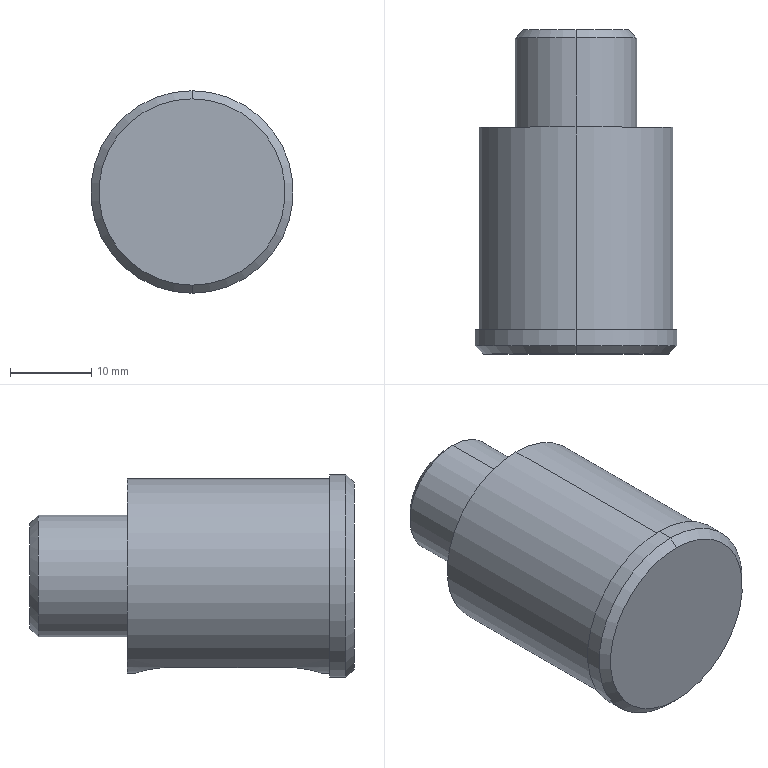Part | SolidWorks | features ICE 3, Chamfer 1, Extrusion 1 | 1 solid | 19 faces | box 25 x 40 x 25 mm | volume 14197 mm3 | cylinder 8 | plane 7 | cone 4 | commonest cylinder face diameters 8 x2 15 x2 24 x2 25 x2
STEP:
#1=CARTESIAN_POINT('',(0.,0.,-11.5));
#2=VERTEX_POINT('',#1);
#3=CARTESIAN_POINT('',(0.,0.,11.5));
#4=VERTEX_POINT('',#3);
#5=CARTESIAN_POINT('',(0.,0.,0.));
#6=DIRECTION('',(0.,-1.,0.));
#7=DIRECTION('',(0.,0.,1.));
#8=AXIS2_PLACEMENT_3D('',#5,#6,#7);
#9=CIRCLE('',#8,11.5);
#10=EDGE_CURVE('',#2,#4,#9,.T.);
#11=ORIENTED_EDGE('',*,*,#10,.F.);
#12=CARTESIAN_POINT('',(0.,1.,-12.5));
#13=VERTEX_POINT('',#12);
#14=CARTESIAN_POINT('',(0.,1.,-12.5));
#15=DIRECTION('',(0.,0.7071,-0.7071));
#16=VECTOR('',#15,1000.);
#17=LINE('',#14,#16);
#18=EDGE_CURVE('',#2,#13,#17,.T.);
#19=ORIENTED_EDGE('',*,*,#18,.T.);
#20=CARTESIAN_POINT('',(0.,1.,12.5));
#21=VERTEX_POINT('',#20);
#22=CARTESIAN_POINT('',(0.,1.,0.));
#23=DIRECTION('',(0.,1.,0.));
#24=DIRECTION('',(0.,0.,1.));
#25=AXIS2_PLACEMENT_3D('',#22,#23,#24);
#26=CIRCLE('',#25,12.5);
#27=EDGE_CURVE('',#21,#13,#26,.T.);
#28=ORIENTED_EDGE('',*,*,#27,.F.);
#29=CARTESIAN_POINT('',(0.,1.,12.5));
#30=DIRECTION('',(0.,0.7071,0.7071));
#31=VECTOR('',#30,1000.);
#32=LINE('',#29,#31);
#33=EDGE_CURVE('',#4,#21,#32,.T.);
#34=ORIENTED_EDGE('',*,*,#33,.F.);
#35=EDGE_LOOP('',(#11,#19,#28,#34));
#36=FACE_OUTER_BOUND('',#35,.T.);
#37=CARTESIAN_POINT('',(0.,1.,0.));
#38=DIRECTION('',(0.,1.,0.));
#39=DIRECTION('',(0.,0.,1.));
#40=AXIS2_PLACEMENT_3D('',#37,#38,#39);
#41=CONICAL_SURFACE('',#40,12.5,0.7854);
#42=ADVANCED_FACE('',(#36),#41,.T.);
#43=CARTESIAN_POINT('',(0.,40.,6.5));
#44=VERTEX_POINT('',#43);
#45=CARTESIAN_POINT('',(0.,40.,-6.5));
#46=VERTEX_POINT('',#45);
#47=CARTESIAN_POINT('',(0.,40.,0.));
#48=DIRECTION('',(0.,1.,0.));
#49=DIRECTION('',(0.,0.,1.));
#50=AXIS2_PLACEMENT_3D('',#47,#48,#49);
#51=CIRCLE('',#50,6.5);
#52=EDGE_CURVE('',#44,#46,#51,.T.);
#53=ORIENTED_EDGE('',*,*,#52,.F.);
#54=CARTESIAN_POINT('',(0.,39.,7.5));
#55=VERTEX_POINT('',#54);
#56=CARTESIAN_POINT('',(0.,40.,6.5));
#57=DIRECTION('',(0.,-0.7071,0.7071));
#58=VECTOR('',#57,1000.);
#59=LINE('',#56,#58);
#60=EDGE_CURVE('',#44,#55,#59,.T.);
#61=ORIENTED_EDGE('',*,*,#60,.T.);
#62=CARTESIAN_POINT('',(0.,39.,-7.5));
#63=VERTEX_POINT('',#62);
#64=CARTESIAN_POINT('',(0.,39.,0.));
#65=DIRECTION('',(0.,-1.,0.));
#66=DIRECTION('',(0.,0.,1.));
#67=AXIS2_PLACEMENT_3D('',#64,#65,#66);
#68=CIRCLE('',#67,7.5);
#69=EDGE_CURVE('',#63,#55,#68,.T.);
#70=ORIENTED_EDGE('',*,*,#69,.F.);
#71=CARTESIAN_POINT('',(0.,40.,-6.5));
#72=DIRECTION('',(0.,-0.7071,-0.7071));
#73=VECTOR('',#72,1000.);
#74=LINE('',#71,#73);
#75=EDGE_CURVE('',#46,#63,#74,.T.);
#76=ORIENTED_EDGE('',*,*,#75,.F.);
#77=EDGE_LOOP('',(#53,#61,#70,#76));
#78=FACE_OUTER_BOUND('',#77,.T.);
#79=CARTESIAN_POINT('',(0.,40.,0.));
#80=DIRECTION('',(0.,-1.,0.));
#81=DIRECTION('',(0.,0.,-1.));
#82=AXIS2_PLACEMENT_3D('',#79,#80,#81);
#83=CONICAL_SURFACE('',#82,6.5,0.7854);
#84=ADVANCED_FACE('',(#78),#83,.T.);
#85=ORIENTED_EDGE('',*,*,#69,.T.);
#86=CARTESIAN_POINT('',(0.,28.,7.5));
#87=VERTEX_POINT('',#86);
#88=CARTESIAN_POINT('',(0.,40.,7.5));
#89=DIRECTION('',(0.,-1.,0.));
#90=VECTOR('',#89,1000.);
#91=LINE('',#88,#90);
#92=EDGE_CURVE('',#55,#87,#91,.T.);
#93=ORIENTED_EDGE('',*,*,#92,.T.);
#94=CARTESIAN_POINT('',(0.,28.,-7.5));
#95=VERTEX_POINT('',#94);
#96=CARTESIAN_POINT('',(0.,28.,0.));
#97=DIRECTION('',(0.,1.,0.));
#98=DIRECTION('',(0.,0.,1.));
#99=AXIS2_PLACEMENT_3D('',#96,#97,#98);
#100=CIRCLE('',#99,7.5);
#101=EDGE_CURVE('',#87,#95,#100,.T.);
#102=ORIENTED_EDGE('',*,*,#101,.T.);
#103=CARTESIAN_POINT('',(0.,40.,-7.5));
#104=DIRECTION('',(0.,-1.,0.));
#105=VECTOR('',#104,1000.);
#106=LINE('',#103,#105);
#107=EDGE_CURVE('',#63,#95,#106,.T.);
#108=ORIENTED_EDGE('',*,*,#107,.F.);
#109=EDGE_LOOP('',(#85,#93,#102,#108));
#110=FACE_OUTER_BOUND('',#109,.T.);
#111=CARTESIAN_POINT('',(0.,40.,0.));
#112=DIRECTION('',(0.,-1.,0.));
#113=DIRECTION('',(0.,0.,-1.));
#114=AXIS2_PLACEMENT_3D('',#111,#112,#113);
#115=CYLINDRICAL_SURFACE('',#114,7.5);
#116=ADVANCED_FACE('',(#110),#115,.T.);
#117=CARTESIAN_POINT('',(0.,28.,12.));
#118=VERTEX_POINT('',#117);
#119=CARTESIAN_POINT('',(0.,28.,-12.));
#120=VERTEX_POINT('',#119);
#121=CARTESIAN_POINT('',(0.,28.,0.));
#122=DIRECTION('',(0.,1.,0.));
#123=DIRECTION('',(0.,0.,1.));
#124=AXIS2_PLACEMENT_3D('',#121,#122,#123);
#125=CIRCLE('',#124,12.);
#126=EDGE_CURVE('',#118,#120,#125,.T.);
#127=ORIENTED_EDGE('',*,*,#126,.F.);
#128=CARTESIAN_POINT('',(0.,3.,12.));
#129=VERTEX_POINT('',#128);
#130=CARTESIAN_POINT('',(0.,28.,12.));
#131=DIRECTION('',(0.,-1.,0.));
#132=VECTOR('',#131,1000.);
#133=LINE('',#130,#132);
#134=EDGE_CURVE('',#118,#129,#133,.T.);
#135=ORIENTED_EDGE('',*,*,#134,.T.);
#136=CARTESIAN_POINT('',(0.,3.,-12.));
#137=VERTEX_POINT('',#136);
#138=CARTESIAN_POINT('',(0.,3.,0.));
#139=DIRECTION('',(0.,1.,0.));
#140=DIRECTION('',(0.,0.,1.));
#141=AXIS2_PLACEMENT_3D('',#138,#139,#140);
#142=CIRCLE('',#141,12.);
#143=EDGE_CURVE('',#129,#137,#142,.T.);
#144=ORIENTED_EDGE('',*,*,#143,.T.);
#145=CARTESIAN_POINT('',(0.,4.,-12.));
#146=VERTEX_POINT('',#145);
#147=CARTESIAN_POINT('',(0.,28.,-12.));
#148=DIRECTION('',(0.,-1.,0.));
#149=VECTOR('',#148,1000.);
#150=LINE('',#147,#149);
#151=EDGE_CURVE('',#146,#137,#150,.T.);
#152=ORIENTED_EDGE('',*,*,#151,.F.);
#153=CARTESIAN_POINT('',(4.,8.,-11.314));
#154=VERTEX_POINT('',#153);
#155=CARTESIAN_POINT('',(0.,4.,-12.));
#156=CARTESIAN_POINT('',(0.2628,4.,-12.));
#157=CARTESIAN_POINT('',(0.5297,4.027,-11.991));
#158=CARTESIAN_POINT('',(1.044,4.13,-11.957));
#159=CARTESIAN_POINT('',(1.294,4.206,-11.933));
#160=CARTESIAN_POINT('',(1.78,4.408,-11.87));
#161=CARTESIAN_POINT('',(2.011,4.533,-11.832));
#162=CARTESIAN_POINT('',(2.442,4.821,-11.751));
#163=CARTESIAN_POINT('',(2.645,4.988,-11.706));
#164=CARTESIAN_POINT('',(3.013,5.356,-11.617));
#165=CARTESIAN_POINT('',(3.177,5.556,-11.573));
#166=CARTESIAN_POINT('',(3.467,5.987,-11.489));
#167=CARTESIAN_POINT('',(3.592,6.221,-11.45));
#168=CARTESIAN_POINT('',(3.792,6.702,-11.385));
#169=CARTESIAN_POINT('',(3.869,6.951,-11.359));
#170=CARTESIAN_POINT('',(3.973,7.468,-11.323));
#171=CARTESIAN_POINT('',(4.,7.734,-11.314));
#172=CARTESIAN_POINT('',(4.,8.,-11.314));
#173=B_SPLINE_CURVE_WITH_KNOTS('',3,(#155,#156,#157,#158,#159,#160,#161,#162,#163,#164,#165,#166,#167,#168,#169,#170,#171,#172),.UNSPECIFIED.,.F.,.F.,(4,2,2,2,2,2,2,2,4),(0.0063,0.007086,0.007873,0.008659,0.009446,0.01023,0.01102,0.01181,0.01259),.UNSPECIFIED.);
#174=EDGE_CURVE('',#146,#154,#173,.T.);
#175=ORIENTED_EDGE('',*,*,#174,.T.);
#176=CARTESIAN_POINT('',(4.,23.,-11.314));
#177=VERTEX_POINT('',#176);
#178=CARTESIAN_POINT('',(4.,28.,-11.314));
#179=DIRECTION('',(0.,1.,0.));
#180=VECTOR('',#179,1000.);
#181=LINE('',#178,#180);
#182=EDGE_CURVE('',#154,#177,#181,.T.);
#183=ORIENTED_EDGE('',*,*,#182,.T.);
#184=CARTESIAN_POINT('',(0.,27.,-12.));
#185=VERTEX_POINT('',#184);
#186=CARTESIAN_POINT('',(4.,23.,-11.314));
#187=CARTESIAN_POINT('',(4.,23.266,-11.314));
#188=CARTESIAN_POINT('',(3.974,23.528,-11.323));
#189=CARTESIAN_POINT('',(3.871,24.042,-11.359));
#190=CARTESIAN_POINT('',(3.793,24.297,-11.385));
#191=CARTESIAN_POINT('',(3.591,24.781,-11.45));
#192=CARTESIAN_POINT('',(3.468,25.01,-11.489));
#193=CARTESIAN_POINT('',(3.178,25.443,-11.573));
#194=CARTESIAN_POINT('',(3.01,25.647,-11.618));
#195=CARTESIAN_POINT('',(2.644,26.013,-11.707));
#196=CARTESIAN_POINT('',(2.444,26.178,-11.751));
#197=CARTESIAN_POINT('',(2.007,26.47,-11.833));
#198=CARTESIAN_POINT('',(1.777,26.593,-11.87));
#199=CARTESIAN_POINT('',(1.296,26.793,-11.932));
#200=CARTESIAN_POINT('',(1.042,26.871,-11.958));
#201=CARTESIAN_POINT('',(0.5242,26.974,-11.991));
#202=CARTESIAN_POINT('',(0.2632,27.,-12.));
#203=CARTESIAN_POINT('',(0.,27.,-12.));
#204=B_SPLINE_CURVE_WITH_KNOTS('',3,(#186,#187,#188,#189,#190,#191,#192,#193,#194,#195,#196,#197,#198,#199,#200,#201,#202,#203),.UNSPECIFIED.,.F.,.F.,(4,2,2,2,2,2,2,2,4),(0.,0.0007875,0.001575,0.002362,0.00315,0.003937,0.004725,0.005512,0.0063),.UNSPECIFIED.);
#205=EDGE_CURVE('',#177,#185,#204,.T.);
#206=ORIENTED_EDGE('',*,*,#205,.T.);
#207=CARTESIAN_POINT('',(0.,28.,-12.));
#208=DIRECTION('',(0.,-1.,0.));
#209=VECTOR('',#208,1000.);
#210=LINE('',#207,#209);
#211=EDGE_CURVE('',#120,#185,#210,.T.);
#212=ORIENTED_EDGE('',*,*,#211,.F.);
#213=EDGE_LOOP('',(#127,#135,#144,#152,#175,#183,#206,#212));
#214=FACE_OUTER_BOUND('',#213,.T.);
#215=CARTESIAN_POINT('',(0.,28.,0.));
#216=DIRECTION('',(0.,-1.,0.));
#217=DIRECTION('',(0.,0.,-1.));
#218=AXIS2_PLACEMENT_3D('',#215,#216,#217);
#219=CYLINDRICAL_SURFACE('',#218,12.);
#220=ADVANCED_FACE('',(#214),#219,.T.);
#221=CARTESIAN_POINT('',(0.,3.,12.5));
#222=VERTEX_POINT('',#221);
#223=CARTESIAN_POINT('',(0.,3.,-12.5));
#224=VERTEX_POINT('',#223);
#225=CARTESIAN_POINT('',(0.,3.,0.));
#226=DIRECTION('',(0.,1.,0.));
#227=DIRECTION('',(0.,0.,1.));
#228=AXIS2_PLACEMENT_3D('',#225,#226,#227);
#229=CIRCLE('',#228,12.5);
#230=EDGE_CURVE('',#222,#224,#229,.T.);
#231=ORIENTED_EDGE('',*,*,#230,.F.);
#232=CARTESIAN_POINT('',(0.,3.,12.5));
#233=DIRECTION('',(0.,-1.,0.));
#234=VECTOR('',#233,1000.);
#235=LINE('',#232,#234);
#236=EDGE_CURVE('',#222,#21,#235,.T.);
#237=ORIENTED_EDGE('',*,*,#236,.T.);
#238=ORIENTED_EDGE('',*,*,#27,.T.);
#239=CARTESIAN_POINT('',(0.,3.,-12.5));
#240=DIRECTION('',(0.,-1.,0.));
#241=VECTOR('',#240,1000.);
#242=LINE('',#239,#241);
#243=EDGE_CURVE('',#224,#13,#242,.T.);
#244=ORIENTED_EDGE('',*,*,#243,.F.);
#245=EDGE_LOOP('',(#231,#237,#238,#244));
#246=FACE_OUTER_BOUND('',#245,.T.);
#247=CARTESIAN_POINT('',(0.,3.,0.));
#248=DIRECTION('',(0.,-1.,0.));
#249=DIRECTION('',(0.,0.,-1.));
#250=AXIS2_PLACEMENT_3D('',#247,#248,#249);
#251=CYLINDRICAL_SURFACE('',#250,12.5);
#252=ADVANCED_FACE('',(#246),#251,.T.);
#253=ORIENTED_EDGE('',*,*,#236,.F.);
#254=CARTESIAN_POINT('',(0.,3.,0.));
#255=DIRECTION('',(0.,1.,0.));
#256=DIRECTION('',(0.,0.,1.));
#257=AXIS2_PLACEMENT_3D('',#254,#255,#256);
#258=CIRCLE('',#257,12.5);
#259=EDGE_CURVE('',#224,#222,#258,.T.);
#260=ORIENTED_EDGE('',*,*,#259,.F.);
#261=ORIENTED_EDGE('',*,*,#243,.T.);
#262=CARTESIAN_POINT('',(0.,1.,0.));
#263=DIRECTION('',(0.,1.,0.));
#264=DIRECTION('',(0.,0.,1.));
#265=AXIS2_PLACEMENT_3D('',#262,#263,#264);
#266=CIRCLE('',#265,12.5);
#267=EDGE_CURVE('',#13,#21,#266,.T.);
#268=ORIENTED_EDGE('',*,*,#267,.T.);
#269=EDGE_LOOP('',(#253,#260,#261,#268));
#270=FACE_OUTER_BOUND('',#269,.T.);
#271=CARTESIAN_POINT('',(0.,3.,0.));
#272=DIRECTION('',(0.,-1.,0.));
#273=DIRECTION('',(0.,0.,-1.));
#274=AXIS2_PLACEMENT_3D('',#271,#272,#273);
#275=CYLINDRICAL_SURFACE('',#274,12.5);
#276=ADVANCED_FACE('',(#270),#275,.T.);
#277=CARTESIAN_POINT('',(0.,3.,0.));
#278=DIRECTION('',(0.,1.,0.));
#279=DIRECTION('',(0.,0.,1.));
#280=AXIS2_PLACEMENT_3D('',#277,#278,#279);
#281=CIRCLE('',#280,12.);
#282=EDGE_CURVE('',#137,#129,#281,.T.);
#283=ORIENTED_EDGE('',*,*,#282,.F.);
#284=ORIENTED_EDGE('',*,*,#143,.F.);
#285=EDGE_LOOP('',(#283,#284));
#286=FACE_BOUND('',#285,.T.);
#287=ORIENTED_EDGE('',*,*,#259,.T.);
#288=ORIENTED_EDGE('',*,*,#230,.T.);
#289=EDGE_LOOP('',(#287,#288));
#290=FACE_OUTER_BOUND('',#289,.T.);
#291=CARTESIAN_POINT('',(0.,3.,0.));
#292=DIRECTION('',(0.,1.,0.));
#293=DIRECTION('',(0.,0.,1.));
#294=AXIS2_PLACEMENT_3D('',#291,#292,#293);
#295=PLANE('',#294);
#296=ADVANCED_FACE('',(#286,#290),#295,.T.);
#297=CARTESIAN_POINT('',(0.,0.,0.));
#298=DIRECTION('',(0.,-1.,0.));
#299=DIRECTION('',(0.,0.,1.));
#300=AXIS2_PLACEMENT_3D('',#297,#298,#299);
#301=CIRCLE('',#300,11.5);
#302=EDGE_CURVE('',#4,#2,#301,.T.);
#303=ORIENTED_EDGE('',*,*,#302,.T.);
#304=ORIENTED_EDGE('',*,*,#10,.T.);
#305=EDGE_LOOP('',(#303,#304));
#306=FACE_OUTER_BOUND('',#305,.T.);
#307=CARTESIAN_POINT('',(0.,0.,0.));
#308=DIRECTION('',(0.,1.,0.));
#309=DIRECTION('',(0.,0.,1.));
#310=AXIS2_PLACEMENT_3D('',#307,#308,#309);
#311=PLANE('',#310);
#312=ADVANCED_FACE('',(#306),#311,.F.);
#313=ORIENTED_EDGE('',*,*,#134,.F.);
#314=CARTESIAN_POINT('',(0.,28.,0.));
#315=DIRECTION('',(0.,1.,0.));
#316=DIRECTION('',(0.,0.,1.));
#317=AXIS2_PLACEMENT_3D('',#314,#315,#316);
#318=CIRCLE('',#317,12.);
#319=EDGE_CURVE('',#120,#118,#318,.T.);
#320=ORIENTED_EDGE('',*,*,#319,.F.);
#321=ORIENTED_EDGE('',*,*,#211,.T.);
#322=CARTESIAN_POINT('',(-4.,23.,-11.314));
#323=VERTEX_POINT('',#322);
#324=CARTESIAN_POINT('',(0.,27.,-12.));
#325=CARTESIAN_POINT('',(-0.2628,27.,-12.));
#326=CARTESIAN_POINT('',(-0.5297,26.973,-11.991));
#327=CARTESIAN_POINT('',(-1.044,26.87,-11.957));
#328=CARTESIAN_POINT('',(-1.294,26.794,-11.933));
#329=CARTESIAN_POINT('',(-1.78,26.592,-11.87));
#330=CARTESIAN_POINT('',(-2.011,26.467,-11.832));
#331=CARTESIAN_POINT('',(-2.442,26.179,-11.751));
#332=CARTESIAN_POINT('',(-2.645,26.012,-11.706));
#333=CARTESIAN_POINT('',(-3.013,25.644,-11.617));
#334=CARTESIAN_POINT('',(-3.177,25.444,-11.573));
#335=CARTESIAN_POINT('',(-3.467,25.013,-11.489));
#336=CARTESIAN_POINT('',(-3.592,24.779,-11.45));
#337=CARTESIAN_POINT('',(-3.792,24.298,-11.385));
#338=CARTESIAN_POINT('',(-3.869,24.049,-11.359));
#339=CARTESIAN_POINT('',(-3.973,23.532,-11.323));
#340=CARTESIAN_POINT('',(-4.,23.266,-11.314));
#341=CARTESIAN_POINT('',(-4.,23.,-11.314));
#342=B_SPLINE_CURVE_WITH_KNOTS('',3,(#324,#325,#326,#327,#328,#329,#330,#331,#332,#333,#334,#335,#336,#337,#338,#339,#340,#341),.UNSPECIFIED.,.F.,.F.,(4,2,2,2,2,2,2,2,4),(0.0063,0.007086,0.007873,0.008659,0.009446,0.01023,0.01102,0.01181,0.01259),.UNSPECIFIED.);
#343=EDGE_CURVE('',#185,#323,#342,.T.);
#344=ORIENTED_EDGE('',*,*,#343,.T.);
#345=CARTESIAN_POINT('',(-4.,8.,-11.314));
#346=VERTEX_POINT('',#345);
#347=CARTESIAN_POINT('',(-4.,28.,-11.314));
#348=DIRECTION('',(0.,-1.,0.));
#349=VECTOR('',#348,1000.);
#350=LINE('',#347,#349);
#351=EDGE_CURVE('',#323,#346,#350,.T.);
#352=ORIENTED_EDGE('',*,*,#351,.T.);
#353=CARTESIAN_POINT('',(-4.,8.,-11.314));
#354=CARTESIAN_POINT('',(-4.,7.734,-11.314));
#355=CARTESIAN_POINT('',(-3.974,7.472,-11.323));
#356=CARTESIAN_POINT('',(-3.871,6.958,-11.359));
#357=CARTESIAN_POINT('',(-3.793,6.703,-11.385));
#358=CARTESIAN_POINT('',(-3.591,6.219,-11.45));
#359=CARTESIAN_POINT('',(-3.468,5.99,-11.489));
#360=CARTESIAN_POINT('',(-3.178,5.557,-11.573));
#361=CARTESIAN_POINT('',(-3.01,5.353,-11.618));
#362=CARTESIAN_POINT('',(-2.644,4.987,-11.707));
#363=CARTESIAN_POINT('',(-2.444,4.822,-11.751));
#364=CARTESIAN_POINT('',(-2.007,4.53,-11.833));
#365=CARTESIAN_POINT('',(-1.777,4.407,-11.87));
#366=CARTESIAN_POINT('',(-1.296,4.207,-11.932));
#367=CARTESIAN_POINT('',(-1.042,4.129,-11.958));
#368=CARTESIAN_POINT('',(-0.5242,4.026,-11.991));
#369=CARTESIAN_POINT('',(-0.2632,4.,-12.));
#370=CARTESIAN_POINT('',(0.,4.,-12.));
#371=B_SPLINE_CURVE_WITH_KNOTS('',3,(#353,#354,#355,#356,#357,#358,#359,#360,#361,#362,#363,#364,#365,#366,#367,#368,#369,#370),.UNSPECIFIED.,.F.,.F.,(4,2,2,2,2,2,2,2,4),(0.,0.0007875,0.001575,0.002362,0.00315,0.003937,0.004725,0.005512,0.0063),.UNSPECIFIED.);
#372=EDGE_CURVE('',#346,#146,#371,.T.);
#373=ORIENTED_EDGE('',*,*,#372,.T.);
#374=ORIENTED_EDGE('',*,*,#151,.T.);
#375=ORIENTED_EDGE('',*,*,#282,.T.);
#376=EDGE_LOOP('',(#313,#320,#321,#344,#352,#373,#374,#375));
#377=FACE_OUTER_BOUND('',#376,.T.);
#378=CARTESIAN_POINT('',(0.,28.,0.));
#379=DIRECTION('',(0.,-1.,0.));
#380=DIRECTION('',(0.,0.,-1.));
#381=AXIS2_PLACEMENT_3D('',#378,#379,#380);
#382=CYLINDRICAL_SURFACE('',#381,12.);
#383=ADVANCED_FACE('',(#377),#382,.T.);
#384=CARTESIAN_POINT('',(0.,28.,0.));
#385=DIRECTION('',(0.,1.,0.));
#386=DIRECTION('',(0.,0.,1.));
#387=AXIS2_PLACEMENT_3D('',#384,#385,#386);
#388=CIRCLE('',#387,7.5);
#389=EDGE_CURVE('',#95,#87,#388,.T.);
#390=ORIENTED_EDGE('',*,*,#389,.F.);
#391=ORIENTED_EDGE('',*,*,#101,.F.);
#392=EDGE_LOOP('',(#390,#391));
#393=FACE_BOUND('',#392,.T.);
#394=ORIENTED_EDGE('',*,*,#319,.T.);
#395=ORIENTED_EDGE('',*,*,#126,.T.);
#396=EDGE_LOOP('',(#394,#395));
#397=FACE_OUTER_BOUND('',#396,.T.);
#398=CARTESIAN_POINT('',(0.,28.,0.));
#399=DIRECTION('',(0.,1.,0.));
#400=DIRECTION('',(0.,0.,1.));
#401=AXIS2_PLACEMENT_3D('',#398,#399,#400);
#402=PLANE('',#401);
#403=ADVANCED_FACE('',(#393,#397),#402,.T.);
#404=ORIENTED_EDGE('',*,*,#92,.F.);
#405=CARTESIAN_POINT('',(0.,39.,0.));
#406=DIRECTION('',(0.,-1.,0.));
#407=DIRECTION('',(0.,0.,1.));
#408=AXIS2_PLACEMENT_3D('',#405,#406,#407);
#409=CIRCLE('',#408,7.5);
#410=EDGE_CURVE('',#55,#63,#409,.T.);
#411=ORIENTED_EDGE('',*,*,#410,.T.);
#412=ORIENTED_EDGE('',*,*,#107,.T.);
#413=ORIENTED_EDGE('',*,*,#389,.T.);
#414=EDGE_LOOP('',(#404,#411,#412,#413));
#415=FACE_OUTER_BOUND('',#414,.T.);
#416=CARTESIAN_POINT('',(0.,40.,0.));
#417=DIRECTION('',(0.,-1.,0.));
#418=DIRECTION('',(0.,0.,-1.));
#419=AXIS2_PLACEMENT_3D('',#416,#417,#418);
#420=CYLINDRICAL_SURFACE('',#419,7.5);
#421=ADVANCED_FACE('',(#415),#420,.T.);
#422=CARTESIAN_POINT('',(0.,40.,0.));
#423=DIRECTION('',(0.,1.,0.));
#424=DIRECTION('',(0.,0.,1.));
#425=AXIS2_PLACEMENT_3D('',#422,#423,#424);
#426=CIRCLE('',#425,6.5);
#427=EDGE_CURVE('',#46,#44,#426,.T.);
#428=ORIENTED_EDGE('',*,*,#427,.T.);
#429=ORIENTED_EDGE('',*,*,#52,.T.);
#430=EDGE_LOOP('',(#428,#429));
#431=FACE_OUTER_BOUND('',#430,.T.);
#432=CARTESIAN_POINT('',(0.,40.,0.));
#433=DIRECTION('',(0.,1.,0.));
#434=DIRECTION('',(0.,0.,1.));
#435=AXIS2_PLACEMENT_3D('',#432,#433,#434);
#436=PLANE('',#435);
#437=ADVANCED_FACE('',(#431),#436,.T.);
#438=CARTESIAN_POINT('',(4.,23.,-8.));
#439=VERTEX_POINT('',#438);
#440=CARTESIAN_POINT('',(4.,23.,-8.));
#441=DIRECTION('',(0.,0.,-1.));
#442=VECTOR('',#441,1000.);
#443=LINE('',#440,#442);
#444=EDGE_CURVE('',#439,#177,#443,.T.);
#445=ORIENTED_EDGE('',*,*,#444,.F.);
#446=CARTESIAN_POINT('',(-4.,23.,-8.));
#447=VERTEX_POINT('',#446);
#448=CARTESIAN_POINT('',(0.,23.,-8.));
#449=DIRECTION('',(0.,0.,-1.));
#450=DIRECTION('',(-1.,0.,0.));
#451=AXIS2_PLACEMENT_3D('',#448,#449,#450);
#452=CIRCLE('',#451,4.);
#453=EDGE_CURVE('',#447,#439,#452,.T.);
#454=ORIENTED_EDGE('',*,*,#453,.F.);
#455=CARTESIAN_POINT('',(-4.,23.,-8.));
#456=DIRECTION('',(0.,0.,-1.));
#457=VECTOR('',#456,1000.);
#458=LINE('',#455,#457);
#459=EDGE_CURVE('',#447,#323,#458,.T.);
#460=ORIENTED_EDGE('',*,*,#459,.T.);
#461=ORIENTED_EDGE('',*,*,#343,.F.);
#462=ORIENTED_EDGE('',*,*,#205,.F.);
#463=EDGE_LOOP('',(#445,#454,#460,#461,#462));
#464=FACE_OUTER_BOUND('',#463,.T.);
#465=CARTESIAN_POINT('',(0.,23.,-8.));
#466=DIRECTION('',(0.,0.,-1.));
#467=DIRECTION('',(-1.,0.,0.));
#468=AXIS2_PLACEMENT_3D('',#465,#466,#467);
#469=CYLINDRICAL_SURFACE('',#468,4.);
#470=ADVANCED_FACE('',(#464),#469,.F.);
#471=ORIENTED_EDGE('',*,*,#459,.F.);
#472=CARTESIAN_POINT('',(-4.,8.,-8.));
#473=VERTEX_POINT('',#472);
#474=CARTESIAN_POINT('',(-4.,23.,-8.));
#475=DIRECTION('',(0.,1.,0.));
#476=VECTOR('',#475,1000.);
#477=LINE('',#474,#476);
#478=EDGE_CURVE('',#473,#447,#477,.T.);
#479=ORIENTED_EDGE('',*,*,#478,.F.);
#480=CARTESIAN_POINT('',(-4.,8.,-8.));
#481=DIRECTION('',(0.,0.,-1.));
#482=VECTOR('',#481,1000.);
#483=LINE('',#480,#482);
#484=EDGE_CURVE('',#473,#346,#483,.T.);
#485=ORIENTED_EDGE('',*,*,#484,.T.);
#486=ORIENTED_EDGE('',*,*,#351,.F.);
#487=EDGE_LOOP('',(#471,#479,#485,#486));
#488=FACE_OUTER_BOUND('',#487,.T.);
#489=CARTESIAN_POINT('',(-4.,23.,-8.));
#490=DIRECTION('',(-1.,0.,0.));
#491=DIRECTION('',(0.,0.,1.));
#492=AXIS2_PLACEMENT_3D('',#489,#490,#491);
#493=PLANE('',#492);
#494=ADVANCED_FACE('',(#488),#493,.F.);
#495=ORIENTED_EDGE('',*,*,#484,.F.);
#496=CARTESIAN_POINT('',(4.,8.,-8.));
#497=VERTEX_POINT('',#496);
#498=CARTESIAN_POINT('',(0.,8.,-8.));
#499=DIRECTION('',(0.,0.,-1.));
#500=DIRECTION('',(-1.,0.,0.));
#501=AXIS2_PLACEMENT_3D('',#498,#499,#500);
#502=CIRCLE('',#501,4.);
#503=EDGE_CURVE('',#497,#473,#502,.T.);
#504=ORIENTED_EDGE('',*,*,#503,.F.);
#505=CARTESIAN_POINT('',(4.,8.,-8.));
#506=DIRECTION('',(0.,0.,-1.));
#507=VECTOR('',#506,1000.);
#508=LINE('',#505,#507);
#509=EDGE_CURVE('',#497,#154,#508,.T.);
#510=ORIENTED_EDGE('',*,*,#509,.T.);
#511=ORIENTED_EDGE('',*,*,#174,.F.);
#512=ORIENTED_EDGE('',*,*,#372,.F.);
#513=EDGE_LOOP('',(#495,#504,#510,#511,#512));
#514=FACE_OUTER_BOUND('',#513,.T.);
#515=CARTESIAN_POINT('',(0.,8.,-8.));
#516=DIRECTION('',(0.,0.,-1.));
#517=DIRECTION('',(-1.,0.,0.));
#518=AXIS2_PLACEMENT_3D('',#515,#516,#517);
#519=CYLINDRICAL_SURFACE('',#518,4.);
#520=ADVANCED_FACE('',(#514),#519,.F.);
#521=ORIENTED_EDGE('',*,*,#509,.F.);
#522=CARTESIAN_POINT('',(4.,23.,-8.));
#523=DIRECTION('',(0.,-1.,0.));
#524=VECTOR('',#523,1000.);
#525=LINE('',#522,#524);
#526=EDGE_CURVE('',#439,#497,#525,.T.);
#527=ORIENTED_EDGE('',*,*,#526,.F.);
#528=ORIENTED_EDGE('',*,*,#444,.T.);
#529=ORIENTED_EDGE('',*,*,#182,.F.);
#530=EDGE_LOOP('',(#521,#527,#528,#529));
#531=FACE_OUTER_BOUND('',#530,.T.);
#532=CARTESIAN_POINT('',(4.,23.,-8.));
#533=DIRECTION('',(1.,0.,0.));
#534=DIRECTION('',(0.,1.,0.));
#535=AXIS2_PLACEMENT_3D('',#532,#533,#534);
#536=PLANE('',#535);
#537=ADVANCED_FACE('',(#531),#536,.F.);
#538=ORIENTED_EDGE('',*,*,#453,.T.);
#539=ORIENTED_EDGE('',*,*,#526,.T.);
#540=ORIENTED_EDGE('',*,*,#503,.T.);
#541=ORIENTED_EDGE('',*,*,#478,.T.);
#542=EDGE_LOOP('',(#538,#539,#540,#541));
#543=FACE_OUTER_BOUND('',#542,.T.);
#544=CARTESIAN_POINT('',(0.,23.,-8.));
#545=DIRECTION('',(0.,0.,-1.));
#546=DIRECTION('',(-1.,0.,0.));
#547=AXIS2_PLACEMENT_3D('',#544,#545,#546);
#548=PLANE('',#547);
#549=ADVANCED_FACE('',(#543),#548,.T.);
#550=ORIENTED_EDGE('',*,*,#60,.F.);
#551=ORIENTED_EDGE('',*,*,#427,.F.);
#552=ORIENTED_EDGE('',*,*,#75,.T.);
#553=ORIENTED_EDGE('',*,*,#410,.F.);
#554=EDGE_LOOP('',(#550,#551,#552,#553));
#555=FACE_OUTER_BOUND('',#554,.T.);
#556=CARTESIAN_POINT('',(0.,40.,0.));
#557=DIRECTION('',(0.,-1.,0.));
#558=DIRECTION('',(0.,0.,-1.));
#559=AXIS2_PLACEMENT_3D('',#556,#557,#558);
#560=CONICAL_SURFACE('',#559,6.5,0.7854);
#561=ADVANCED_FACE('',(#555),#560,.T.);
#562=ORIENTED_EDGE('',*,*,#18,.F.);
#563=ORIENTED_EDGE('',*,*,#302,.F.);
#564=ORIENTED_EDGE('',*,*,#33,.T.);
#565=ORIENTED_EDGE('',*,*,#267,.F.);
#566=EDGE_LOOP('',(#562,#563,#564,#565));
#567=FACE_OUTER_BOUND('',#566,.T.);
#568=CARTESIAN_POINT('',(0.,1.,0.));
#569=DIRECTION('',(0.,1.,0.));
#570=DIRECTION('',(0.,0.,1.));
#571=AXIS2_PLACEMENT_3D('',#568,#569,#570);
#572=CONICAL_SURFACE('',#571,12.5,0.7854);
#573=ADVANCED_FACE('',(#567),#572,.T.);
#574=CLOSED_SHELL('',(#42,#84,#116,#220,#252,#276,#296,#312,#383,#403,#421,#437,#470,#494,#520,#537,#549,#561,#573));
#575=MANIFOLD_SOLID_BREP('',#574);
#576=CARTESIAN_POINT('',(0.,0.,0.));
#577=DIRECTION('',(0.,0.,1.));
#578=DIRECTION('',(1.,0.,0.));
#579=AXIS2_PLACEMENT_3D('',#576,#577,#578);
#580=(LENGTH_UNIT()NAMED_UNIT(*)SI_UNIT(.MILLI.,.METRE.));
#581=UNCERTAINTY_MEASURE_WITH_UNIT(LENGTH_MEASURE(0.00001),#580,'','');
#582=(NAMED_UNIT(*)PLANE_ANGLE_UNIT()SI_UNIT($,.RADIAN.));
#583=(NAMED_UNIT(*)SI_UNIT($,.STERADIAN.)SOLID_ANGLE_UNIT());
#584=(GEOMETRIC_REPRESENTATION_CONTEXT(3)GLOBAL_UNCERTAINTY_ASSIGNED_CONTEXT((#581))GLOBAL_UNIT_ASSIGNED_CONTEXT((#580,#582,#583))REPRESENTATION_CONTEXT('',''));
#585=ADVANCED_BREP_SHAPE_REPRESENTATION('',(#575,#579),#584);